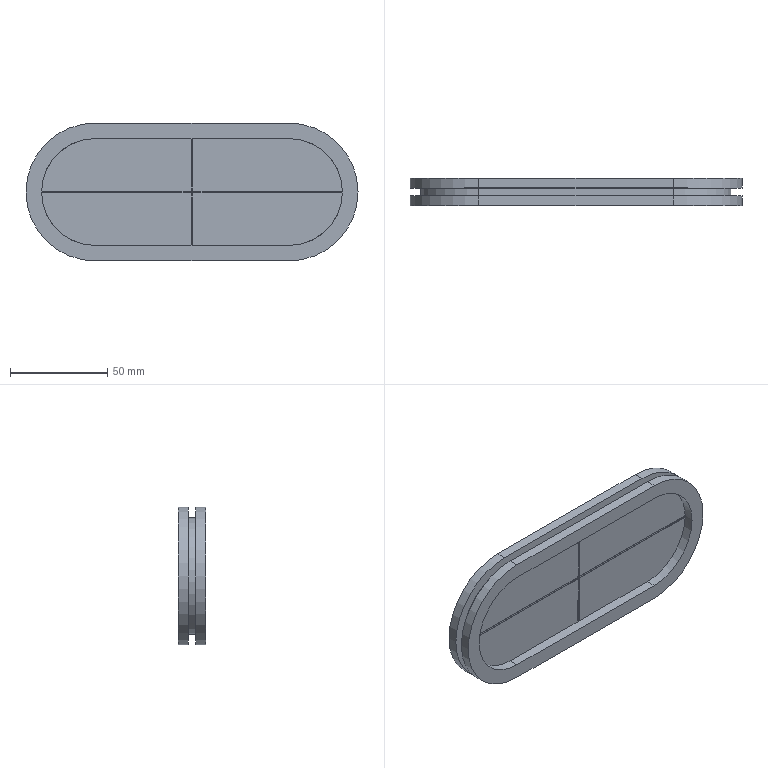Part | SolidWorks | features BaseBody 1 | 1 solid | 54 faces | box 171 x 14 x 71 mm | volume 67060 mm3 | plane 44 | cylinder 10 | commonest cylinder face diameters 55 x4 71 x4 60 x2